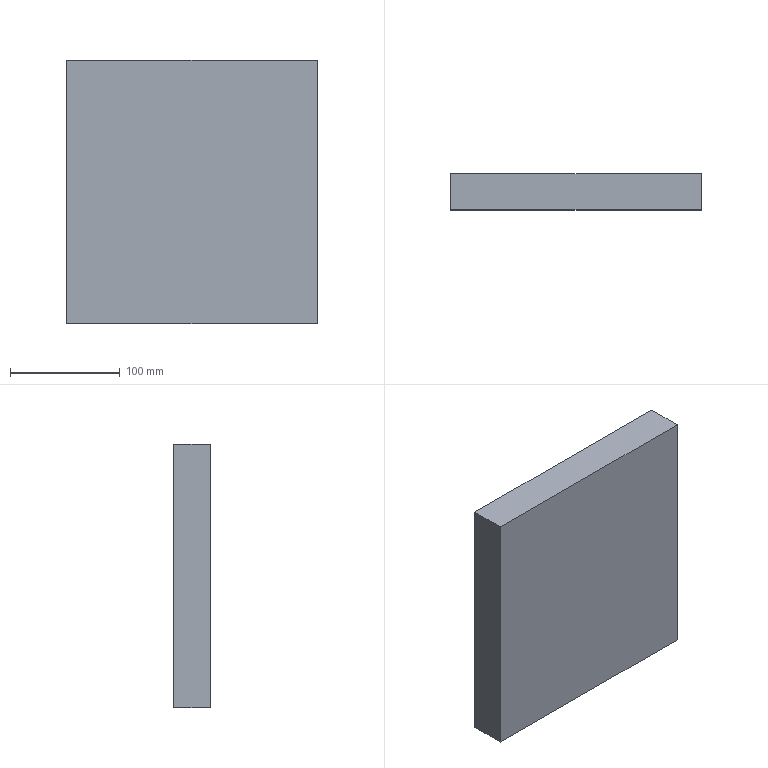Part | NX | 1 solid | 6 faces | box 228 x 33 x 240 mm | volume 1805760 mm3 | plane 6
STEP:
#1=CARTESIAN_POINT('',(-7.326,-727.347,2245.086));
#2=VERTEX_POINT('',#1);
#3=CARTESIAN_POINT('',(-7.326,-760.347,2245.086));
#4=VERTEX_POINT('',#3);
#5=CARTESIAN_POINT('',(-7.326,-727.347,2245.086));
#6=DIRECTION('',(0.,-1.,0.));
#7=VECTOR('',#6,1.);
#8=LINE('',#5,#7);
#9=EDGE_CURVE('',#2,#4,#8,.T.);
#10=ORIENTED_EDGE('',*,*,#9,.T.);
#11=CARTESIAN_POINT('',(-235.326,-760.347,2245.086));
#12=VERTEX_POINT('',#11);
#13=CARTESIAN_POINT('',(-187.326,-760.347,2245.086));
#14=DIRECTION('',(1.,0.,0.));
#15=VECTOR('',#14,1.);
#16=LINE('',#13,#15);
#17=EDGE_CURVE('',#12,#4,#16,.T.);
#18=ORIENTED_EDGE('',*,*,#17,.F.);
#19=CARTESIAN_POINT('',(-235.326,-727.347,2245.086));
#20=VERTEX_POINT('',#19);
#21=CARTESIAN_POINT('',(-235.326,-727.347,2245.086));
#22=DIRECTION('',(0.,-1.,0.));
#23=VECTOR('',#22,1.);
#24=LINE('',#21,#23);
#25=EDGE_CURVE('',#20,#12,#24,.T.);
#26=ORIENTED_EDGE('',*,*,#25,.F.);
#27=CARTESIAN_POINT('',(-187.326,-727.347,2245.086));
#28=DIRECTION('',(1.,0.,0.));
#29=VECTOR('',#28,1.);
#30=LINE('',#27,#29);
#31=EDGE_CURVE('',#20,#2,#30,.T.);
#32=ORIENTED_EDGE('',*,*,#31,.T.);
#33=EDGE_LOOP('',(#10,#18,#26,#32));
#34=FACE_OUTER_BOUND('',#33,.T.);
#35=CARTESIAN_POINT('',(-187.326,-727.347,2245.086));
#36=DIRECTION('',(0.,0.,1.));
#37=DIRECTION('',(0.,-1.,0.));
#38=AXIS2_PLACEMENT_3D('',#35,#36,#37);
#39=PLANE('',#38);
#40=ADVANCED_FACE('',(#34),#39,.F.);
#41=CARTESIAN_POINT('',(-7.326,-760.347,2485.086));
#42=VERTEX_POINT('',#41);
#43=CARTESIAN_POINT('',(-7.326,-760.347,2245.086));
#44=DIRECTION('',(0.,0.,1.));
#45=VECTOR('',#44,1.);
#46=LINE('',#43,#45);
#47=EDGE_CURVE('',#4,#42,#46,.T.);
#48=ORIENTED_EDGE('',*,*,#47,.T.);
#49=CARTESIAN_POINT('',(-235.326,-760.347,2485.086));
#50=VERTEX_POINT('',#49);
#51=CARTESIAN_POINT('',(-187.326,-760.347,2485.086));
#52=DIRECTION('',(1.,0.,0.));
#53=VECTOR('',#52,1.);
#54=LINE('',#51,#53);
#55=EDGE_CURVE('',#50,#42,#54,.T.);
#56=ORIENTED_EDGE('',*,*,#55,.F.);
#57=CARTESIAN_POINT('',(-235.326,-760.347,2245.086));
#58=DIRECTION('',(0.,0.,1.));
#59=VECTOR('',#58,1.);
#60=LINE('',#57,#59);
#61=EDGE_CURVE('',#12,#50,#60,.T.);
#62=ORIENTED_EDGE('',*,*,#61,.F.);
#63=ORIENTED_EDGE('',*,*,#17,.T.);
#64=EDGE_LOOP('',(#48,#56,#62,#63));
#65=FACE_OUTER_BOUND('',#64,.T.);
#66=CARTESIAN_POINT('',(-187.326,-760.347,2245.086));
#67=DIRECTION('',(0.,1.,0.));
#68=DIRECTION('',(0.,0.,1.));
#69=AXIS2_PLACEMENT_3D('',#66,#67,#68);
#70=PLANE('',#69);
#71=ADVANCED_FACE('',(#65),#70,.F.);
#72=CARTESIAN_POINT('',(-7.326,-727.347,2485.086));
#73=VERTEX_POINT('',#72);
#74=CARTESIAN_POINT('',(-7.326,-727.347,2485.086));
#75=DIRECTION('',(0.,1.,0.));
#76=VECTOR('',#75,1.);
#77=LINE('',#74,#76);
#78=EDGE_CURVE('',#42,#73,#77,.T.);
#79=ORIENTED_EDGE('',*,*,#78,.T.);
#80=CARTESIAN_POINT('',(-235.326,-727.347,2485.086));
#81=VERTEX_POINT('',#80);
#82=CARTESIAN_POINT('',(-187.326,-727.347,2485.086));
#83=DIRECTION('',(1.,0.,0.));
#84=VECTOR('',#83,1.);
#85=LINE('',#82,#84);
#86=EDGE_CURVE('',#81,#73,#85,.T.);
#87=ORIENTED_EDGE('',*,*,#86,.F.);
#88=CARTESIAN_POINT('',(-235.326,-760.347,2485.086));
#89=DIRECTION('',(0.,1.,0.));
#90=VECTOR('',#89,1.);
#91=LINE('',#88,#90);
#92=EDGE_CURVE('',#50,#81,#91,.T.);
#93=ORIENTED_EDGE('',*,*,#92,.F.);
#94=ORIENTED_EDGE('',*,*,#55,.T.);
#95=EDGE_LOOP('',(#79,#87,#93,#94));
#96=FACE_OUTER_BOUND('',#95,.T.);
#97=CARTESIAN_POINT('',(-187.326,-727.347,2485.086));
#98=DIRECTION('',(0.,0.,-1.));
#99=DIRECTION('',(-1.,0.,0.));
#100=AXIS2_PLACEMENT_3D('',#97,#98,#99);
#101=PLANE('',#100);
#102=ADVANCED_FACE('',(#96),#101,.F.);
#103=CARTESIAN_POINT('',(-7.326,-727.347,2245.086));
#104=DIRECTION('',(0.,0.,-1.));
#105=VECTOR('',#104,1.);
#106=LINE('',#103,#105);
#107=EDGE_CURVE('',#73,#2,#106,.T.);
#108=ORIENTED_EDGE('',*,*,#107,.T.);
#109=ORIENTED_EDGE('',*,*,#31,.F.);
#110=CARTESIAN_POINT('',(-235.326,-727.347,2485.086));
#111=DIRECTION('',(0.,0.,-1.));
#112=VECTOR('',#111,1.);
#113=LINE('',#110,#112);
#114=EDGE_CURVE('',#81,#20,#113,.T.);
#115=ORIENTED_EDGE('',*,*,#114,.F.);
#116=ORIENTED_EDGE('',*,*,#86,.T.);
#117=EDGE_LOOP('',(#108,#109,#115,#116));
#118=FACE_OUTER_BOUND('',#117,.T.);
#119=CARTESIAN_POINT('',(-187.326,-727.347,2245.086));
#120=DIRECTION('',(0.,-1.,0.));
#121=DIRECTION('',(0.,0.,-1.));
#122=AXIS2_PLACEMENT_3D('',#119,#120,#121);
#123=PLANE('',#122);
#124=ADVANCED_FACE('',(#118),#123,.F.);
#125=ORIENTED_EDGE('',*,*,#9,.F.);
#126=ORIENTED_EDGE('',*,*,#107,.F.);
#127=ORIENTED_EDGE('',*,*,#78,.F.);
#128=ORIENTED_EDGE('',*,*,#47,.F.);
#129=EDGE_LOOP('',(#125,#126,#127,#128));
#130=FACE_OUTER_BOUND('',#129,.T.);
#131=CARTESIAN_POINT('',(-7.326,-760.347,2245.086));
#132=DIRECTION('',(-1.,0.,0.));
#133=DIRECTION('',(0.,0.,1.));
#134=AXIS2_PLACEMENT_3D('',#131,#132,#133);
#135=PLANE('',#134);
#136=ADVANCED_FACE('',(#130),#135,.F.);
#137=ORIENTED_EDGE('',*,*,#114,.T.);
#138=ORIENTED_EDGE('',*,*,#25,.T.);
#139=ORIENTED_EDGE('',*,*,#61,.T.);
#140=ORIENTED_EDGE('',*,*,#92,.T.);
#141=EDGE_LOOP('',(#137,#138,#139,#140));
#142=FACE_OUTER_BOUND('',#141,.T.);
#143=CARTESIAN_POINT('',(-235.326,-727.347,2485.086));
#144=DIRECTION('',(1.,0.,0.));
#145=DIRECTION('',(0.,0.,-1.));
#146=AXIS2_PLACEMENT_3D('',#143,#144,#145);
#147=PLANE('',#146);
#148=ADVANCED_FACE('',(#142),#147,.F.);
#149=CLOSED_SHELL('',(#40,#71,#102,#124,#136,#148));
#150=MANIFOLD_SOLID_BREP('',#149);
#151=(LENGTH_UNIT()NAMED_UNIT(*)SI_UNIT(.MILLI.,.METRE.));
#152=UNCERTAINTY_MEASURE_WITH_UNIT(LENGTH_MEASURE(0.00002),#151,'','');
#153=(NAMED_UNIT(*)PLANE_ANGLE_UNIT()SI_UNIT($,.RADIAN.));
#154=PLANE_ANGLE_MEASURE_WITH_UNIT(PLANE_ANGLE_MEASURE(0.01745),#153);
#155=DIMENSIONAL_EXPONENTS(0.,0.,0.,0.,0.,0.,0.);
#156=(CONVERSION_BASED_UNIT('DEGREE',#154)NAMED_UNIT(#155)PLANE_ANGLE_UNIT());
#157=(NAMED_UNIT(*)SI_UNIT($,.STERADIAN.)SOLID_ANGLE_UNIT());
#158=(GEOMETRIC_REPRESENTATION_CONTEXT(3)GLOBAL_UNCERTAINTY_ASSIGNED_CONTEXT((#152))GLOBAL_UNIT_ASSIGNED_CONTEXT((#151,#156,#157))REPRESENTATION_CONTEXT('',''));
#159=ADVANCED_BREP_SHAPE_REPRESENTATION('',(#150),#158);